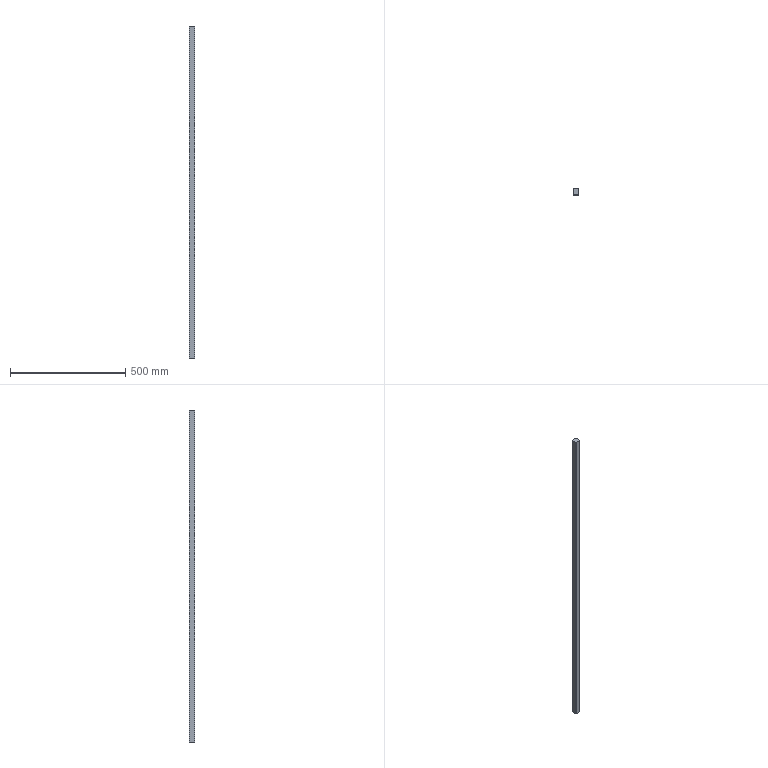Part | SolidWorks | features Extrusion 1 | 1 solid | 10 faces | box 24 x 24 x 1440 mm | volume 829131 mm3 | plane 6 | cylinder 4 | commonest cylinder face diameters 1 x4
STEP:
#1=CARTESIAN_POINT('',(-11.5,12.,-720.));
#2=VERTEX_POINT('',#1);
#3=CARTESIAN_POINT('',(-12.,11.5,-720.));
#4=VERTEX_POINT('',#3);
#5=CARTESIAN_POINT('',(-11.5,11.5,-720.));
#6=DIRECTION('',(0.,0.,1.));
#7=DIRECTION('',(-1.,0.,0.));
#8=AXIS2_PLACEMENT_3D('',#5,#6,#7);
#9=CIRCLE('',#8,0.5);
#10=EDGE_CURVE('',#2,#4,#9,.T.);
#11=ORIENTED_EDGE('',*,*,#10,.T.);
#12=CARTESIAN_POINT('',(-12.,11.5,720.));
#13=VERTEX_POINT('',#12);
#14=CARTESIAN_POINT('',(-12.,11.5,720.));
#15=DIRECTION('',(0.,0.,-1.));
#16=VECTOR('',#15,1000.);
#17=LINE('',#14,#16);
#18=EDGE_CURVE('',#13,#4,#17,.T.);
#19=ORIENTED_EDGE('',*,*,#18,.F.);
#20=CARTESIAN_POINT('',(-11.5,12.,720.));
#21=VERTEX_POINT('',#20);
#22=CARTESIAN_POINT('',(-11.5,11.5,720.));
#23=DIRECTION('',(0.,0.,1.));
#24=DIRECTION('',(-1.,0.,0.));
#25=AXIS2_PLACEMENT_3D('',#22,#23,#24);
#26=CIRCLE('',#25,0.5);
#27=EDGE_CURVE('',#21,#13,#26,.T.);
#28=ORIENTED_EDGE('',*,*,#27,.F.);
#29=CARTESIAN_POINT('',(-11.5,12.,720.));
#30=DIRECTION('',(0.,0.,-1.));
#31=VECTOR('',#30,1000.);
#32=LINE('',#29,#31);
#33=EDGE_CURVE('',#21,#2,#32,.T.);
#34=ORIENTED_EDGE('',*,*,#33,.T.);
#35=EDGE_LOOP('',(#11,#19,#28,#34));
#36=FACE_OUTER_BOUND('',#35,.T.);
#37=CARTESIAN_POINT('',(-11.5,11.5,720.));
#38=DIRECTION('',(0.,0.,-1.));
#39=DIRECTION('',(-1.,0.,0.));
#40=AXIS2_PLACEMENT_3D('',#37,#38,#39);
#41=CYLINDRICAL_SURFACE('',#40,0.5);
#42=ADVANCED_FACE('',(#36),#41,.T.);
#43=CARTESIAN_POINT('',(-12.,-11.5,-720.));
#44=VERTEX_POINT('',#43);
#45=CARTESIAN_POINT('',(-12.,-11.5,-720.));
#46=DIRECTION('',(0.,-1.,0.));
#47=VECTOR('',#46,1000.);
#48=LINE('',#45,#47);
#49=EDGE_CURVE('',#4,#44,#48,.T.);
#50=ORIENTED_EDGE('',*,*,#49,.T.);
#51=CARTESIAN_POINT('',(-12.,-11.5,720.));
#52=VERTEX_POINT('',#51);
#53=CARTESIAN_POINT('',(-12.,-11.5,720.));
#54=DIRECTION('',(0.,0.,-1.));
#55=VECTOR('',#54,1000.);
#56=LINE('',#53,#55);
#57=EDGE_CURVE('',#52,#44,#56,.T.);
#58=ORIENTED_EDGE('',*,*,#57,.F.);
#59=CARTESIAN_POINT('',(-12.,-11.5,720.));
#60=DIRECTION('',(0.,-1.,0.));
#61=VECTOR('',#60,1000.);
#62=LINE('',#59,#61);
#63=EDGE_CURVE('',#13,#52,#62,.T.);
#64=ORIENTED_EDGE('',*,*,#63,.F.);
#65=ORIENTED_EDGE('',*,*,#18,.T.);
#66=EDGE_LOOP('',(#50,#58,#64,#65));
#67=FACE_OUTER_BOUND('',#66,.T.);
#68=CARTESIAN_POINT('',(-12.,-11.5,720.));
#69=DIRECTION('',(1.,0.,0.));
#70=DIRECTION('',(0.,0.,-1.));
#71=AXIS2_PLACEMENT_3D('',#68,#69,#70);
#72=PLANE('',#71);
#73=ADVANCED_FACE('',(#67),#72,.F.);
#74=CARTESIAN_POINT('',(-11.5,-12.,-720.));
#75=VERTEX_POINT('',#74);
#76=CARTESIAN_POINT('',(-11.5,-11.5,-720.));
#77=DIRECTION('',(0.,0.,1.));
#78=DIRECTION('',(-1.,0.,0.));
#79=AXIS2_PLACEMENT_3D('',#76,#77,#78);
#80=CIRCLE('',#79,0.5);
#81=EDGE_CURVE('',#44,#75,#80,.T.);
#82=ORIENTED_EDGE('',*,*,#81,.T.);
#83=CARTESIAN_POINT('',(-11.5,-12.,720.));
#84=VERTEX_POINT('',#83);
#85=CARTESIAN_POINT('',(-11.5,-12.,720.));
#86=DIRECTION('',(0.,0.,-1.));
#87=VECTOR('',#86,1000.);
#88=LINE('',#85,#87);
#89=EDGE_CURVE('',#84,#75,#88,.T.);
#90=ORIENTED_EDGE('',*,*,#89,.F.);
#91=CARTESIAN_POINT('',(-11.5,-11.5,720.));
#92=DIRECTION('',(0.,0.,1.));
#93=DIRECTION('',(-1.,0.,0.));
#94=AXIS2_PLACEMENT_3D('',#91,#92,#93);
#95=CIRCLE('',#94,0.5);
#96=EDGE_CURVE('',#52,#84,#95,.T.);
#97=ORIENTED_EDGE('',*,*,#96,.F.);
#98=ORIENTED_EDGE('',*,*,#57,.T.);
#99=EDGE_LOOP('',(#82,#90,#97,#98));
#100=FACE_OUTER_BOUND('',#99,.T.);
#101=CARTESIAN_POINT('',(-11.5,-11.5,720.));
#102=DIRECTION('',(0.,0.,-1.));
#103=DIRECTION('',(-1.,0.,0.));
#104=AXIS2_PLACEMENT_3D('',#101,#102,#103);
#105=CYLINDRICAL_SURFACE('',#104,0.5);
#106=ADVANCED_FACE('',(#100),#105,.T.);
#107=CARTESIAN_POINT('',(11.5,-12.,-720.));
#108=VERTEX_POINT('',#107);
#109=CARTESIAN_POINT('',(-11.5,-12.,-720.));
#110=DIRECTION('',(1.,0.,0.));
#111=VECTOR('',#110,1000.);
#112=LINE('',#109,#111);
#113=EDGE_CURVE('',#75,#108,#112,.T.);
#114=ORIENTED_EDGE('',*,*,#113,.T.);
#115=CARTESIAN_POINT('',(11.5,-12.,720.));
#116=VERTEX_POINT('',#115);
#117=CARTESIAN_POINT('',(11.5,-12.,720.));
#118=DIRECTION('',(0.,0.,-1.));
#119=VECTOR('',#118,1000.);
#120=LINE('',#117,#119);
#121=EDGE_CURVE('',#116,#108,#120,.T.);
#122=ORIENTED_EDGE('',*,*,#121,.F.);
#123=CARTESIAN_POINT('',(-11.5,-12.,720.));
#124=DIRECTION('',(1.,0.,0.));
#125=VECTOR('',#124,1000.);
#126=LINE('',#123,#125);
#127=EDGE_CURVE('',#84,#116,#126,.T.);
#128=ORIENTED_EDGE('',*,*,#127,.F.);
#129=ORIENTED_EDGE('',*,*,#89,.T.);
#130=EDGE_LOOP('',(#114,#122,#128,#129));
#131=FACE_OUTER_BOUND('',#130,.T.);
#132=CARTESIAN_POINT('',(-11.5,-12.,720.));
#133=DIRECTION('',(0.,1.,0.));
#134=DIRECTION('',(0.,0.,1.));
#135=AXIS2_PLACEMENT_3D('',#132,#133,#134);
#136=PLANE('',#135);
#137=ADVANCED_FACE('',(#131),#136,.F.);
#138=CARTESIAN_POINT('',(12.,-11.5,-720.));
#139=VERTEX_POINT('',#138);
#140=CARTESIAN_POINT('',(11.5,-11.5,-720.));
#141=DIRECTION('',(0.,0.,1.));
#142=DIRECTION('',(1.,0.,0.));
#143=AXIS2_PLACEMENT_3D('',#140,#141,#142);
#144=CIRCLE('',#143,0.5);
#145=EDGE_CURVE('',#108,#139,#144,.T.);
#146=ORIENTED_EDGE('',*,*,#145,.T.);
#147=CARTESIAN_POINT('',(12.,-11.5,720.));
#148=VERTEX_POINT('',#147);
#149=CARTESIAN_POINT('',(12.,-11.5,720.));
#150=DIRECTION('',(0.,0.,-1.));
#151=VECTOR('',#150,1000.);
#152=LINE('',#149,#151);
#153=EDGE_CURVE('',#148,#139,#152,.T.);
#154=ORIENTED_EDGE('',*,*,#153,.F.);
#155=CARTESIAN_POINT('',(11.5,-11.5,720.));
#156=DIRECTION('',(0.,0.,1.));
#157=DIRECTION('',(1.,0.,0.));
#158=AXIS2_PLACEMENT_3D('',#155,#156,#157);
#159=CIRCLE('',#158,0.5);
#160=EDGE_CURVE('',#116,#148,#159,.T.);
#161=ORIENTED_EDGE('',*,*,#160,.F.);
#162=ORIENTED_EDGE('',*,*,#121,.T.);
#163=EDGE_LOOP('',(#146,#154,#161,#162));
#164=FACE_OUTER_BOUND('',#163,.T.);
#165=CARTESIAN_POINT('',(11.5,-11.5,720.));
#166=DIRECTION('',(0.,0.,-1.));
#167=DIRECTION('',(-1.,0.,0.));
#168=AXIS2_PLACEMENT_3D('',#165,#166,#167);
#169=CYLINDRICAL_SURFACE('',#168,0.5);
#170=ADVANCED_FACE('',(#164),#169,.T.);
#171=CARTESIAN_POINT('',(12.,11.5,-720.));
#172=VERTEX_POINT('',#171);
#173=CARTESIAN_POINT('',(12.,-11.5,-720.));
#174=DIRECTION('',(0.,1.,0.));
#175=VECTOR('',#174,1000.);
#176=LINE('',#173,#175);
#177=EDGE_CURVE('',#139,#172,#176,.T.);
#178=ORIENTED_EDGE('',*,*,#177,.T.);
#179=CARTESIAN_POINT('',(12.,11.5,720.));
#180=VERTEX_POINT('',#179);
#181=CARTESIAN_POINT('',(12.,11.5,720.));
#182=DIRECTION('',(0.,0.,-1.));
#183=VECTOR('',#182,1000.);
#184=LINE('',#181,#183);
#185=EDGE_CURVE('',#180,#172,#184,.T.);
#186=ORIENTED_EDGE('',*,*,#185,.F.);
#187=CARTESIAN_POINT('',(12.,-11.5,720.));
#188=DIRECTION('',(0.,1.,0.));
#189=VECTOR('',#188,1000.);
#190=LINE('',#187,#189);
#191=EDGE_CURVE('',#148,#180,#190,.T.);
#192=ORIENTED_EDGE('',*,*,#191,.F.);
#193=ORIENTED_EDGE('',*,*,#153,.T.);
#194=EDGE_LOOP('',(#178,#186,#192,#193));
#195=FACE_OUTER_BOUND('',#194,.T.);
#196=CARTESIAN_POINT('',(12.,-11.5,720.));
#197=DIRECTION('',(-1.,0.,0.));
#198=DIRECTION('',(0.,0.,1.));
#199=AXIS2_PLACEMENT_3D('',#196,#197,#198);
#200=PLANE('',#199);
#201=ADVANCED_FACE('',(#195),#200,.F.);
#202=CARTESIAN_POINT('',(11.5,12.,-720.));
#203=VERTEX_POINT('',#202);
#204=CARTESIAN_POINT('',(11.5,11.5,-720.));
#205=DIRECTION('',(0.,0.,1.));
#206=DIRECTION('',(-1.,0.,0.));
#207=AXIS2_PLACEMENT_3D('',#204,#205,#206);
#208=CIRCLE('',#207,0.5);
#209=EDGE_CURVE('',#172,#203,#208,.T.);
#210=ORIENTED_EDGE('',*,*,#209,.T.);
#211=CARTESIAN_POINT('',(11.5,12.,720.));
#212=VERTEX_POINT('',#211);
#213=CARTESIAN_POINT('',(11.5,12.,720.));
#214=DIRECTION('',(0.,0.,-1.));
#215=VECTOR('',#214,1000.);
#216=LINE('',#213,#215);
#217=EDGE_CURVE('',#212,#203,#216,.T.);
#218=ORIENTED_EDGE('',*,*,#217,.F.);
#219=CARTESIAN_POINT('',(11.5,11.5,720.));
#220=DIRECTION('',(0.,0.,1.));
#221=DIRECTION('',(-1.,0.,0.));
#222=AXIS2_PLACEMENT_3D('',#219,#220,#221);
#223=CIRCLE('',#222,0.5);
#224=EDGE_CURVE('',#180,#212,#223,.T.);
#225=ORIENTED_EDGE('',*,*,#224,.F.);
#226=ORIENTED_EDGE('',*,*,#185,.T.);
#227=EDGE_LOOP('',(#210,#218,#225,#226));
#228=FACE_OUTER_BOUND('',#227,.T.);
#229=CARTESIAN_POINT('',(11.5,11.5,720.));
#230=DIRECTION('',(0.,0.,-1.));
#231=DIRECTION('',(-1.,0.,0.));
#232=AXIS2_PLACEMENT_3D('',#229,#230,#231);
#233=CYLINDRICAL_SURFACE('',#232,0.5);
#234=ADVANCED_FACE('',(#228),#233,.T.);
#235=CARTESIAN_POINT('',(-11.5,12.,-720.));
#236=DIRECTION('',(-1.,0.,0.));
#237=VECTOR('',#236,1000.);
#238=LINE('',#235,#237);
#239=EDGE_CURVE('',#203,#2,#238,.T.);
#240=ORIENTED_EDGE('',*,*,#239,.T.);
#241=ORIENTED_EDGE('',*,*,#33,.F.);
#242=CARTESIAN_POINT('',(-11.5,12.,720.));
#243=DIRECTION('',(-1.,0.,0.));
#244=VECTOR('',#243,1000.);
#245=LINE('',#242,#244);
#246=EDGE_CURVE('',#212,#21,#245,.T.);
#247=ORIENTED_EDGE('',*,*,#246,.F.);
#248=ORIENTED_EDGE('',*,*,#217,.T.);
#249=EDGE_LOOP('',(#240,#241,#247,#248));
#250=FACE_OUTER_BOUND('',#249,.T.);
#251=CARTESIAN_POINT('',(-11.5,12.,720.));
#252=DIRECTION('',(0.,-1.,0.));
#253=DIRECTION('',(0.,0.,-1.));
#254=AXIS2_PLACEMENT_3D('',#251,#252,#253);
#255=PLANE('',#254);
#256=ADVANCED_FACE('',(#250),#255,.F.);
#257=ORIENTED_EDGE('',*,*,#27,.T.);
#258=ORIENTED_EDGE('',*,*,#63,.T.);
#259=ORIENTED_EDGE('',*,*,#96,.T.);
#260=ORIENTED_EDGE('',*,*,#127,.T.);
#261=ORIENTED_EDGE('',*,*,#160,.T.);
#262=ORIENTED_EDGE('',*,*,#191,.T.);
#263=ORIENTED_EDGE('',*,*,#224,.T.);
#264=ORIENTED_EDGE('',*,*,#246,.T.);
#265=EDGE_LOOP('',(#257,#258,#259,#260,#261,#262,#263,#264));
#266=FACE_OUTER_BOUND('',#265,.T.);
#267=CARTESIAN_POINT('',(-11.5,11.5,720.));
#268=DIRECTION('',(0.,0.,-1.));
#269=DIRECTION('',(-1.,0.,0.));
#270=AXIS2_PLACEMENT_3D('',#267,#268,#269);
#271=PLANE('',#270);
#272=ADVANCED_FACE('',(#266),#271,.F.);
#273=ORIENTED_EDGE('',*,*,#10,.F.);
#274=ORIENTED_EDGE('',*,*,#239,.F.);
#275=ORIENTED_EDGE('',*,*,#209,.F.);
#276=ORIENTED_EDGE('',*,*,#177,.F.);
#277=ORIENTED_EDGE('',*,*,#145,.F.);
#278=ORIENTED_EDGE('',*,*,#113,.F.);
#279=ORIENTED_EDGE('',*,*,#81,.F.);
#280=ORIENTED_EDGE('',*,*,#49,.F.);
#281=EDGE_LOOP('',(#273,#274,#275,#276,#277,#278,#279,#280));
#282=FACE_OUTER_BOUND('',#281,.T.);
#283=CARTESIAN_POINT('',(-11.5,11.5,-720.));
#284=DIRECTION('',(0.,0.,-1.));
#285=DIRECTION('',(-1.,0.,0.));
#286=AXIS2_PLACEMENT_3D('',#283,#284,#285);
#287=PLANE('',#286);
#288=ADVANCED_FACE('',(#282),#287,.T.);
#289=CLOSED_SHELL('',(#42,#73,#106,#137,#170,#201,#234,#256,#272,#288));
#290=MANIFOLD_SOLID_BREP('',#289);
#291=CARTESIAN_POINT('',(0.,0.,0.));
#292=DIRECTION('',(0.,0.,1.));
#293=DIRECTION('',(1.,0.,0.));
#294=AXIS2_PLACEMENT_3D('',#291,#292,#293);
#295=(LENGTH_UNIT()NAMED_UNIT(*)SI_UNIT(.MILLI.,.METRE.));
#296=UNCERTAINTY_MEASURE_WITH_UNIT(LENGTH_MEASURE(0.00001),#295,'','');
#297=(NAMED_UNIT(*)PLANE_ANGLE_UNIT()SI_UNIT($,.RADIAN.));
#298=(NAMED_UNIT(*)SI_UNIT($,.STERADIAN.)SOLID_ANGLE_UNIT());
#299=(GEOMETRIC_REPRESENTATION_CONTEXT(3)GLOBAL_UNCERTAINTY_ASSIGNED_CONTEXT((#296))GLOBAL_UNIT_ASSIGNED_CONTEXT((#295,#297,#298))REPRESENTATION_CONTEXT('',''));
#300=ADVANCED_BREP_SHAPE_REPRESENTATION('',(#290,#294),#299);